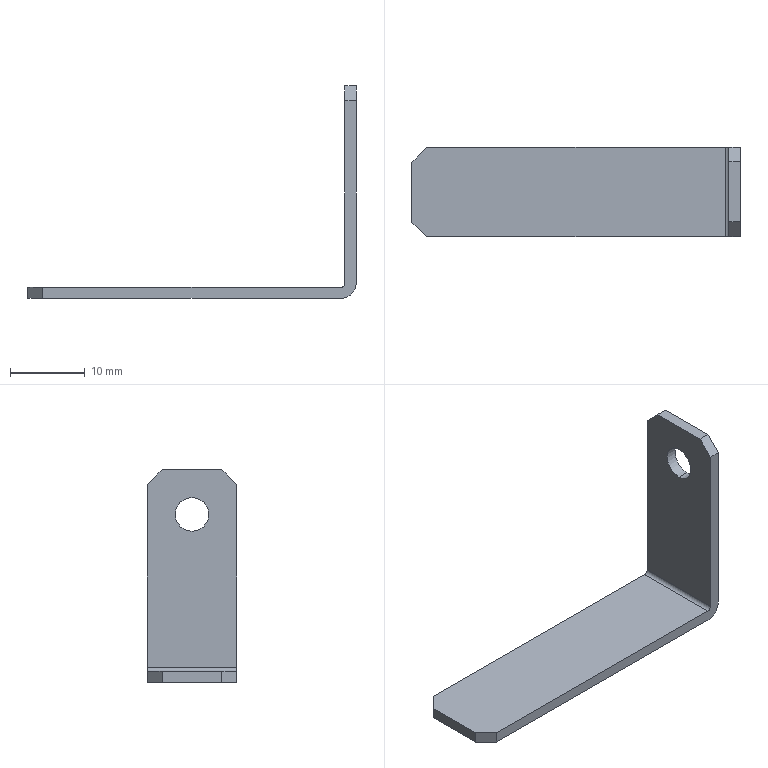Part | SolidWorks | features Fillet 2, Chamfer 1, Extrusion 1, ICE 1 | 1 solid | 16 faces | box 44 x 12 x 28.5 mm | volume 1232 mm3 | plane 12 | cylinder 4 | commonest cylinder face diameters 4.5 x2 1 x1 4 x1
STEP:
#1=CARTESIAN_POINT('',(-1.5,6.,-3.75));
#2=VERTEX_POINT('',#1);
#3=CARTESIAN_POINT('',(-1.5,6.,-8.25));
#4=VERTEX_POINT('',#3);
#5=CARTESIAN_POINT('',(-1.5,6.,-6.));
#6=DIRECTION('',(1.,0.,0.));
#7=DIRECTION('',(0.,0.,-1.));
#8=AXIS2_PLACEMENT_3D('',#5,#6,#7);
#9=CIRCLE('',#8,2.25);
#10=EDGE_CURVE('',#2,#4,#9,.T.);
#11=ORIENTED_EDGE('',*,*,#10,.F.);
#12=CARTESIAN_POINT('',(0.,6.,-3.75));
#13=VERTEX_POINT('',#12);
#14=CARTESIAN_POINT('',(-44.,6.,-3.75));
#15=DIRECTION('',(1.,0.,0.));
#16=VECTOR('',#15,1000.);
#17=LINE('',#14,#16);
#18=EDGE_CURVE('',#2,#13,#17,.T.);
#19=ORIENTED_EDGE('',*,*,#18,.T.);
#20=CARTESIAN_POINT('',(0.,6.,-8.25));
#21=VERTEX_POINT('',#20);
#22=CARTESIAN_POINT('',(0.,6.,-6.));
#23=DIRECTION('',(1.,0.,0.));
#24=DIRECTION('',(0.,0.,-1.));
#25=AXIS2_PLACEMENT_3D('',#22,#23,#24);
#26=CIRCLE('',#25,2.25);
#27=EDGE_CURVE('',#13,#21,#26,.T.);
#28=ORIENTED_EDGE('',*,*,#27,.T.);
#29=CARTESIAN_POINT('',(-44.,6.,-8.25));
#30=DIRECTION('',(1.,0.,0.));
#31=VECTOR('',#30,1000.);
#32=LINE('',#29,#31);
#33=EDGE_CURVE('',#4,#21,#32,.T.);
#34=ORIENTED_EDGE('',*,*,#33,.F.);
#35=EDGE_LOOP('',(#11,#19,#28,#34));
#36=FACE_OUTER_BOUND('',#35,.T.);
#37=CARTESIAN_POINT('',(-44.,6.,-6.));
#38=DIRECTION('',(1.,0.,0.));
#39=DIRECTION('',(0.,0.,-1.));
#40=AXIS2_PLACEMENT_3D('',#37,#38,#39);
#41=CYLINDRICAL_SURFACE('',#40,2.25);
#42=ADVANCED_FACE('',(#36),#41,.F.);
#43=CARTESIAN_POINT('',(0.,6.,-6.));
#44=DIRECTION('',(1.,0.,0.));
#45=DIRECTION('',(0.,0.,-1.));
#46=AXIS2_PLACEMENT_3D('',#43,#44,#45);
#47=CIRCLE('',#46,2.25);
#48=EDGE_CURVE('',#21,#13,#47,.T.);
#49=ORIENTED_EDGE('',*,*,#48,.F.);
#50=ORIENTED_EDGE('',*,*,#27,.F.);
#51=EDGE_LOOP('',(#49,#50));
#52=FACE_BOUND('',#51,.T.);
#53=CARTESIAN_POINT('',(0.,0.,-2.));
#54=VERTEX_POINT('',#53);
#55=CARTESIAN_POINT('',(0.,0.,-26.5));
#56=VERTEX_POINT('',#55);
#57=CARTESIAN_POINT('',(0.,0.,0.));
#58=DIRECTION('',(0.,0.,-1.));
#59=VECTOR('',#58,1000.);
#60=LINE('',#57,#59);
#61=EDGE_CURVE('',#54,#56,#60,.T.);
#62=ORIENTED_EDGE('',*,*,#61,.T.);
#63=CARTESIAN_POINT('',(0.,12.,-26.5));
#64=VERTEX_POINT('',#63);
#65=CARTESIAN_POINT('',(0.,12.,-26.5));
#66=DIRECTION('',(0.,1.,0.));
#67=VECTOR('',#66,1000.);
#68=LINE('',#65,#67);
#69=EDGE_CURVE('',#56,#64,#68,.T.);
#70=ORIENTED_EDGE('',*,*,#69,.T.);
#71=CARTESIAN_POINT('',(0.,12.,-2.));
#72=VERTEX_POINT('',#71);
#73=CARTESIAN_POINT('',(0.,12.,0.));
#74=DIRECTION('',(0.,0.,-1.));
#75=VECTOR('',#74,1000.);
#76=LINE('',#73,#75);
#77=EDGE_CURVE('',#72,#64,#76,.T.);
#78=ORIENTED_EDGE('',*,*,#77,.F.);
#79=CARTESIAN_POINT('',(0.,10.,0.));
#80=VERTEX_POINT('',#79);
#81=CARTESIAN_POINT('',(0.,12.,-2.));
#82=DIRECTION('',(0.,-0.7071,0.7071));
#83=VECTOR('',#82,1000.);
#84=LINE('',#81,#83);
#85=EDGE_CURVE('',#72,#80,#84,.T.);
#86=ORIENTED_EDGE('',*,*,#85,.T.);
#87=CARTESIAN_POINT('',(0.,2.,0.));
#88=VERTEX_POINT('',#87);
#89=CARTESIAN_POINT('',(0.,12.,0.));
#90=DIRECTION('',(0.,-1.,0.));
#91=VECTOR('',#90,1000.);
#92=LINE('',#89,#91);
#93=EDGE_CURVE('',#80,#88,#92,.T.);
#94=ORIENTED_EDGE('',*,*,#93,.T.);
#95=CARTESIAN_POINT('',(0.,2.,0.));
#96=DIRECTION('',(0.,-0.7071,-0.7071));
#97=VECTOR('',#96,1000.);
#98=LINE('',#95,#97);
#99=EDGE_CURVE('',#88,#54,#98,.T.);
#100=ORIENTED_EDGE('',*,*,#99,.T.);
#101=EDGE_LOOP('',(#62,#70,#78,#86,#94,#100));
#102=FACE_OUTER_BOUND('',#101,.T.);
#103=CARTESIAN_POINT('',(0.,12.,0.));
#104=DIRECTION('',(-1.,0.,0.));
#105=DIRECTION('',(0.,0.,1.));
#106=AXIS2_PLACEMENT_3D('',#103,#104,#105);
#107=PLANE('',#106);
#108=ADVANCED_FACE('',(#52,#102),#107,.F.);
#109=CARTESIAN_POINT('',(-2.,12.,-28.5));
#110=VERTEX_POINT('',#109);
#111=CARTESIAN_POINT('',(-42.,12.,-28.5));
#112=VERTEX_POINT('',#111);
#113=CARTESIAN_POINT('',(0.,12.,-28.5));
#114=DIRECTION('',(-1.,0.,0.));
#115=VECTOR('',#114,1000.);
#116=LINE('',#113,#115);
#117=EDGE_CURVE('',#110,#112,#116,.T.);
#118=ORIENTED_EDGE('',*,*,#117,.F.);
#119=CARTESIAN_POINT('',(-2.,0.,-28.5));
#120=VERTEX_POINT('',#119);
#121=CARTESIAN_POINT('',(-2.,12.,-28.5));
#122=DIRECTION('',(0.,-1.,0.));
#123=VECTOR('',#122,1000.);
#124=LINE('',#121,#123);
#125=EDGE_CURVE('',#110,#120,#124,.T.);
#126=ORIENTED_EDGE('',*,*,#125,.T.);
#127=CARTESIAN_POINT('',(-42.,0.,-28.5));
#128=VERTEX_POINT('',#127);
#129=CARTESIAN_POINT('',(0.,0.,-28.5));
#130=DIRECTION('',(-1.,0.,0.));
#131=VECTOR('',#130,1000.);
#132=LINE('',#129,#131);
#133=EDGE_CURVE('',#120,#128,#132,.T.);
#134=ORIENTED_EDGE('',*,*,#133,.T.);
#135=CARTESIAN_POINT('',(-44.,2.,-28.5));
#136=VERTEX_POINT('',#135);
#137=CARTESIAN_POINT('',(-44.,2.,-28.5));
#138=DIRECTION('',(-0.7071,0.7071,0.));
#139=VECTOR('',#138,1000.);
#140=LINE('',#137,#139);
#141=EDGE_CURVE('',#128,#136,#140,.T.);
#142=ORIENTED_EDGE('',*,*,#141,.T.);
#143=CARTESIAN_POINT('',(-44.,10.,-28.5));
#144=VERTEX_POINT('',#143);
#145=CARTESIAN_POINT('',(-44.,12.,-28.5));
#146=DIRECTION('',(0.,-1.,0.));
#147=VECTOR('',#146,1000.);
#148=LINE('',#145,#147);
#149=EDGE_CURVE('',#144,#136,#148,.T.);
#150=ORIENTED_EDGE('',*,*,#149,.F.);
#151=CARTESIAN_POINT('',(-42.,12.,-28.5));
#152=DIRECTION('',(0.7071,0.7071,0.));
#153=VECTOR('',#152,1000.);
#154=LINE('',#151,#153);
#155=EDGE_CURVE('',#144,#112,#154,.T.);
#156=ORIENTED_EDGE('',*,*,#155,.T.);
#157=EDGE_LOOP('',(#118,#126,#134,#142,#150,#156));
#158=FACE_OUTER_BOUND('',#157,.T.);
#159=CARTESIAN_POINT('',(0.,12.,-28.5));
#160=DIRECTION('',(0.,0.,1.));
#161=DIRECTION('',(1.,0.,0.));
#162=AXIS2_PLACEMENT_3D('',#159,#160,#161);
#163=PLANE('',#162);
#164=ADVANCED_FACE('',(#158),#163,.F.);
#165=ORIENTED_EDGE('',*,*,#149,.T.);
#166=CARTESIAN_POINT('',(-44.,2.,-27.));
#167=VERTEX_POINT('',#166);
#168=CARTESIAN_POINT('',(-44.,2.,-27.));
#169=DIRECTION('',(0.,0.,1.));
#170=VECTOR('',#169,1000.);
#171=LINE('',#168,#170);
#172=EDGE_CURVE('',#136,#167,#171,.T.);
#173=ORIENTED_EDGE('',*,*,#172,.T.);
#174=CARTESIAN_POINT('',(-44.,10.,-27.));
#175=VERTEX_POINT('',#174);
#176=CARTESIAN_POINT('',(-44.,12.,-27.));
#177=DIRECTION('',(0.,-1.,0.));
#178=VECTOR('',#177,1000.);
#179=LINE('',#176,#178);
#180=EDGE_CURVE('',#175,#167,#179,.T.);
#181=ORIENTED_EDGE('',*,*,#180,.F.);
#182=CARTESIAN_POINT('',(-44.,10.,-28.5));
#183=DIRECTION('',(0.,0.,-1.));
#184=VECTOR('',#183,1000.);
#185=LINE('',#182,#184);
#186=EDGE_CURVE('',#175,#144,#185,.T.);
#187=ORIENTED_EDGE('',*,*,#186,.T.);
#188=EDGE_LOOP('',(#165,#173,#181,#187));
#189=FACE_OUTER_BOUND('',#188,.T.);
#190=CARTESIAN_POINT('',(-44.,12.,-27.));
#191=DIRECTION('',(1.,0.,0.));
#192=DIRECTION('',(0.,0.,-1.));
#193=AXIS2_PLACEMENT_3D('',#190,#191,#192);
#194=PLANE('',#193);
#195=ADVANCED_FACE('',(#189),#194,.F.);
#196=CARTESIAN_POINT('',(-42.,0.,-27.));
#197=VERTEX_POINT('',#196);
#198=CARTESIAN_POINT('',(-2.,0.,-27.));
#199=VERTEX_POINT('',#198);
#200=CARTESIAN_POINT('',(-44.,0.,-27.));
#201=DIRECTION('',(1.,0.,0.));
#202=VECTOR('',#201,1000.);
#203=LINE('',#200,#202);
#204=EDGE_CURVE('',#197,#199,#203,.T.);
#205=ORIENTED_EDGE('',*,*,#204,.T.);
#206=CARTESIAN_POINT('',(-2.,12.,-27.));
#207=VERTEX_POINT('',#206);
#208=CARTESIAN_POINT('',(-2.,12.,-27.));
#209=DIRECTION('',(0.,1.,0.));
#210=VECTOR('',#209,1000.);
#211=LINE('',#208,#210);
#212=EDGE_CURVE('',#199,#207,#211,.T.);
#213=ORIENTED_EDGE('',*,*,#212,.T.);
#214=CARTESIAN_POINT('',(-42.,12.,-27.));
#215=VERTEX_POINT('',#214);
#216=CARTESIAN_POINT('',(-44.,12.,-27.));
#217=DIRECTION('',(1.,0.,0.));
#218=VECTOR('',#217,1000.);
#219=LINE('',#216,#218);
#220=EDGE_CURVE('',#215,#207,#219,.T.);
#221=ORIENTED_EDGE('',*,*,#220,.F.);
#222=CARTESIAN_POINT('',(-42.,12.,-27.));
#223=DIRECTION('',(-0.7071,-0.7071,0.));
#224=VECTOR('',#223,1000.);
#225=LINE('',#222,#224);
#226=EDGE_CURVE('',#215,#175,#225,.T.);
#227=ORIENTED_EDGE('',*,*,#226,.T.);
#228=ORIENTED_EDGE('',*,*,#180,.T.);
#229=CARTESIAN_POINT('',(-44.,2.,-27.));
#230=DIRECTION('',(0.7071,-0.7071,0.));
#231=VECTOR('',#230,1000.);
#232=LINE('',#229,#231);
#233=EDGE_CURVE('',#167,#197,#232,.T.);
#234=ORIENTED_EDGE('',*,*,#233,.T.);
#235=EDGE_LOOP('',(#205,#213,#221,#227,#228,#234));
#236=FACE_OUTER_BOUND('',#235,.T.);
#237=CARTESIAN_POINT('',(-44.,12.,-27.));
#238=DIRECTION('',(0.,0.,-1.));
#239=DIRECTION('',(-1.,0.,0.));
#240=AXIS2_PLACEMENT_3D('',#237,#238,#239);
#241=PLANE('',#240);
#242=ADVANCED_FACE('',(#236),#241,.F.);
#243=CARTESIAN_POINT('',(-1.5,6.,-6.));
#244=DIRECTION('',(1.,0.,0.));
#245=DIRECTION('',(0.,0.,-1.));
#246=AXIS2_PLACEMENT_3D('',#243,#244,#245);
#247=CIRCLE('',#246,2.25);
#248=EDGE_CURVE('',#4,#2,#247,.T.);
#249=ORIENTED_EDGE('',*,*,#248,.T.);
#250=ORIENTED_EDGE('',*,*,#10,.T.);
#251=EDGE_LOOP('',(#249,#250));
#252=FACE_BOUND('',#251,.T.);
#253=CARTESIAN_POINT('',(-1.5,12.,-26.5));
#254=VERTEX_POINT('',#253);
#255=CARTESIAN_POINT('',(-1.5,12.,-2.));
#256=VERTEX_POINT('',#255);
#257=CARTESIAN_POINT('',(-1.5,12.,0.));
#258=DIRECTION('',(0.,0.,1.));
#259=VECTOR('',#258,1000.);
#260=LINE('',#257,#259);
#261=EDGE_CURVE('',#254,#256,#260,.T.);
#262=ORIENTED_EDGE('',*,*,#261,.F.);
#263=CARTESIAN_POINT('',(-1.5,0.,-26.5));
#264=VERTEX_POINT('',#263);
#265=CARTESIAN_POINT('',(-1.5,0.,-26.5));
#266=DIRECTION('',(0.,-1.,0.));
#267=VECTOR('',#266,1000.);
#268=LINE('',#265,#267);
#269=EDGE_CURVE('',#254,#264,#268,.T.);
#270=ORIENTED_EDGE('',*,*,#269,.T.);
#271=CARTESIAN_POINT('',(-1.5,0.,-2.));
#272=VERTEX_POINT('',#271);
#273=CARTESIAN_POINT('',(-1.5,0.,0.));
#274=DIRECTION('',(0.,0.,1.));
#275=VECTOR('',#274,1000.);
#276=LINE('',#273,#275);
#277=EDGE_CURVE('',#264,#272,#276,.T.);
#278=ORIENTED_EDGE('',*,*,#277,.T.);
#279=CARTESIAN_POINT('',(-1.5,2.,0.));
#280=VERTEX_POINT('',#279);
#281=CARTESIAN_POINT('',(-1.5,2.,0.));
#282=DIRECTION('',(0.,0.7071,0.7071));
#283=VECTOR('',#282,1000.);
#284=LINE('',#281,#283);
#285=EDGE_CURVE('',#272,#280,#284,.T.);
#286=ORIENTED_EDGE('',*,*,#285,.T.);
#287=CARTESIAN_POINT('',(-1.5,10.,0.));
#288=VERTEX_POINT('',#287);
#289=CARTESIAN_POINT('',(-1.5,12.,0.));
#290=DIRECTION('',(0.,-1.,0.));
#291=VECTOR('',#290,1000.);
#292=LINE('',#289,#291);
#293=EDGE_CURVE('',#288,#280,#292,.T.);
#294=ORIENTED_EDGE('',*,*,#293,.F.);
#295=CARTESIAN_POINT('',(-1.5,12.,-2.));
#296=DIRECTION('',(0.,0.7071,-0.7071));
#297=VECTOR('',#296,1000.);
#298=LINE('',#295,#297);
#299=EDGE_CURVE('',#288,#256,#298,.T.);
#300=ORIENTED_EDGE('',*,*,#299,.T.);
#301=EDGE_LOOP('',(#262,#270,#278,#286,#294,#300));
#302=FACE_OUTER_BOUND('',#301,.T.);
#303=CARTESIAN_POINT('',(-1.5,12.,0.));
#304=DIRECTION('',(1.,0.,0.));
#305=DIRECTION('',(0.,0.,-1.));
#306=AXIS2_PLACEMENT_3D('',#303,#304,#305);
#307=PLANE('',#306);
#308=ADVANCED_FACE('',(#252,#302),#307,.F.);
#309=ORIENTED_EDGE('',*,*,#293,.T.);
#310=CARTESIAN_POINT('',(0.,2.,0.));
#311=DIRECTION('',(1.,0.,0.));
#312=VECTOR('',#311,1000.);
#313=LINE('',#310,#312);
#314=EDGE_CURVE('',#280,#88,#313,.T.);
#315=ORIENTED_EDGE('',*,*,#314,.T.);
#316=ORIENTED_EDGE('',*,*,#93,.F.);
#317=CARTESIAN_POINT('',(-1.5,10.,0.));
#318=DIRECTION('',(-1.,0.,0.));
#319=VECTOR('',#318,1000.);
#320=LINE('',#317,#319);
#321=EDGE_CURVE('',#80,#288,#320,.T.);
#322=ORIENTED_EDGE('',*,*,#321,.T.);
#323=EDGE_LOOP('',(#309,#315,#316,#322));
#324=FACE_OUTER_BOUND('',#323,.T.);
#325=CARTESIAN_POINT('',(0.,12.,0.));
#326=DIRECTION('',(0.,0.,-1.));
#327=DIRECTION('',(-1.,0.,0.));
#328=AXIS2_PLACEMENT_3D('',#325,#326,#327);
#329=PLANE('',#328);
#330=ADVANCED_FACE('',(#324),#329,.F.);
#331=ORIENTED_EDGE('',*,*,#77,.T.);
#332=CARTESIAN_POINT('',(-2.,12.,-26.5));
#333=DIRECTION('',(0.,1.,0.));
#334=DIRECTION('',(0.,0.,1.));
#335=AXIS2_PLACEMENT_3D('',#332,#333,#334);
#336=CIRCLE('',#335,2.);
#337=EDGE_CURVE('',#64,#110,#336,.T.);
#338=ORIENTED_EDGE('',*,*,#337,.T.);
#339=ORIENTED_EDGE('',*,*,#117,.T.);
#340=CARTESIAN_POINT('',(-42.,12.,-27.));
#341=DIRECTION('',(0.,0.,1.));
#342=VECTOR('',#341,1000.);
#343=LINE('',#340,#342);
#344=EDGE_CURVE('',#112,#215,#343,.T.);
#345=ORIENTED_EDGE('',*,*,#344,.T.);
#346=ORIENTED_EDGE('',*,*,#220,.T.);
#347=CARTESIAN_POINT('',(-2.,12.,-26.5));
#348=DIRECTION('',(0.,-1.,0.));
#349=DIRECTION('',(0.,0.,1.));
#350=AXIS2_PLACEMENT_3D('',#347,#348,#349);
#351=CIRCLE('',#350,0.5);
#352=EDGE_CURVE('',#207,#254,#351,.T.);
#353=ORIENTED_EDGE('',*,*,#352,.T.);
#354=ORIENTED_EDGE('',*,*,#261,.T.);
#355=CARTESIAN_POINT('',(0.,12.,-2.));
#356=DIRECTION('',(1.,0.,0.));
#357=VECTOR('',#356,1000.);
#358=LINE('',#355,#357);
#359=EDGE_CURVE('',#256,#72,#358,.T.);
#360=ORIENTED_EDGE('',*,*,#359,.T.);
#361=EDGE_LOOP('',(#331,#338,#339,#345,#346,#353,#354,#360));
#362=FACE_OUTER_BOUND('',#361,.T.);
#363=CARTESIAN_POINT('',(0.,12.,0.));
#364=DIRECTION('',(0.,1.,0.));
#365=DIRECTION('',(0.,0.,1.));
#366=AXIS2_PLACEMENT_3D('',#363,#364,#365);
#367=PLANE('',#366);
#368=ADVANCED_FACE('',(#362),#367,.T.);
#369=ORIENTED_EDGE('',*,*,#133,.F.);
#370=CARTESIAN_POINT('',(-2.,0.,-26.5));
#371=DIRECTION('',(0.,-1.,0.));
#372=DIRECTION('',(0.,0.,1.));
#373=AXIS2_PLACEMENT_3D('',#370,#371,#372);
#374=CIRCLE('',#373,2.);
#375=EDGE_CURVE('',#120,#56,#374,.T.);
#376=ORIENTED_EDGE('',*,*,#375,.T.);
#377=ORIENTED_EDGE('',*,*,#61,.F.);
#378=CARTESIAN_POINT('',(0.,0.,-2.));
#379=DIRECTION('',(-1.,0.,0.));
#380=VECTOR('',#379,1000.);
#381=LINE('',#378,#380);
#382=EDGE_CURVE('',#54,#272,#381,.T.);
#383=ORIENTED_EDGE('',*,*,#382,.T.);
#384=ORIENTED_EDGE('',*,*,#277,.F.);
#385=CARTESIAN_POINT('',(-2.,0.,-26.5));
#386=DIRECTION('',(0.,1.,0.));
#387=DIRECTION('',(0.,0.,1.));
#388=AXIS2_PLACEMENT_3D('',#385,#386,#387);
#389=CIRCLE('',#388,0.5);
#390=EDGE_CURVE('',#264,#199,#389,.T.);
#391=ORIENTED_EDGE('',*,*,#390,.T.);
#392=ORIENTED_EDGE('',*,*,#204,.F.);
#393=CARTESIAN_POINT('',(-42.,0.,0.));
#394=DIRECTION('',(0.,0.,-1.));
#395=VECTOR('',#394,1000.);
#396=LINE('',#393,#395);
#397=EDGE_CURVE('',#197,#128,#396,.T.);
#398=ORIENTED_EDGE('',*,*,#397,.T.);
#399=EDGE_LOOP('',(#369,#376,#377,#383,#384,#391,#392,#398));
#400=FACE_OUTER_BOUND('',#399,.T.);
#401=CARTESIAN_POINT('',(0.,0.,0.));
#402=DIRECTION('',(0.,1.,0.));
#403=DIRECTION('',(0.,0.,1.));
#404=AXIS2_PLACEMENT_3D('',#401,#402,#403);
#405=PLANE('',#404);
#406=ADVANCED_FACE('',(#400),#405,.F.);
#407=ORIENTED_EDGE('',*,*,#18,.F.);
#408=ORIENTED_EDGE('',*,*,#248,.F.);
#409=ORIENTED_EDGE('',*,*,#33,.T.);
#410=ORIENTED_EDGE('',*,*,#48,.T.);
#411=EDGE_LOOP('',(#407,#408,#409,#410));
#412=FACE_OUTER_BOUND('',#411,.T.);
#413=CARTESIAN_POINT('',(-44.,6.,-6.));
#414=DIRECTION('',(1.,0.,0.));
#415=DIRECTION('',(0.,0.,-1.));
#416=AXIS2_PLACEMENT_3D('',#413,#414,#415);
#417=CYLINDRICAL_SURFACE('',#416,2.25);
#418=ADVANCED_FACE('',(#412),#417,.F.);
#419=ORIENTED_EDGE('',*,*,#141,.F.);
#420=ORIENTED_EDGE('',*,*,#397,.F.);
#421=ORIENTED_EDGE('',*,*,#233,.F.);
#422=ORIENTED_EDGE('',*,*,#172,.F.);
#423=EDGE_LOOP('',(#419,#420,#421,#422));
#424=FACE_OUTER_BOUND('',#423,.T.);
#425=CARTESIAN_POINT('',(-44.,2.,-27.));
#426=DIRECTION('',(0.7071,0.7071,0.));
#427=DIRECTION('',(0.,0.,1.));
#428=AXIS2_PLACEMENT_3D('',#425,#426,#427);
#429=PLANE('',#428);
#430=ADVANCED_FACE('',(#424),#429,.F.);
#431=ORIENTED_EDGE('',*,*,#155,.F.);
#432=ORIENTED_EDGE('',*,*,#186,.F.);
#433=ORIENTED_EDGE('',*,*,#226,.F.);
#434=ORIENTED_EDGE('',*,*,#344,.F.);
#435=EDGE_LOOP('',(#431,#432,#433,#434));
#436=FACE_OUTER_BOUND('',#435,.T.);
#437=CARTESIAN_POINT('',(-42.,12.,0.));
#438=DIRECTION('',(-0.7071,0.7071,0.));
#439=DIRECTION('',(0.,0.,-1.));
#440=AXIS2_PLACEMENT_3D('',#437,#438,#439);
#441=PLANE('',#440);
#442=ADVANCED_FACE('',(#436),#441,.T.);
#443=ORIENTED_EDGE('',*,*,#285,.F.);
#444=ORIENTED_EDGE('',*,*,#382,.F.);
#445=ORIENTED_EDGE('',*,*,#99,.F.);
#446=ORIENTED_EDGE('',*,*,#314,.F.);
#447=EDGE_LOOP('',(#443,#444,#445,#446));
#448=FACE_OUTER_BOUND('',#447,.T.);
#449=CARTESIAN_POINT('',(0.,2.,0.));
#450=DIRECTION('',(0.,0.7071,-0.7071));
#451=DIRECTION('',(1.,0.,0.));
#452=AXIS2_PLACEMENT_3D('',#449,#450,#451);
#453=PLANE('',#452);
#454=ADVANCED_FACE('',(#448),#453,.F.);
#455=ORIENTED_EDGE('',*,*,#299,.F.);
#456=ORIENTED_EDGE('',*,*,#321,.F.);
#457=ORIENTED_EDGE('',*,*,#85,.F.);
#458=ORIENTED_EDGE('',*,*,#359,.F.);
#459=EDGE_LOOP('',(#455,#456,#457,#458));
#460=FACE_OUTER_BOUND('',#459,.T.);
#461=CARTESIAN_POINT('',(0.,12.,-2.));
#462=DIRECTION('',(0.,0.7071,0.7071));
#463=DIRECTION('',(-1.,0.,0.));
#464=AXIS2_PLACEMENT_3D('',#461,#462,#463);
#465=PLANE('',#464);
#466=ADVANCED_FACE('',(#460),#465,.T.);
#467=ORIENTED_EDGE('',*,*,#337,.F.);
#468=ORIENTED_EDGE('',*,*,#69,.F.);
#469=ORIENTED_EDGE('',*,*,#375,.F.);
#470=ORIENTED_EDGE('',*,*,#125,.F.);
#471=EDGE_LOOP('',(#467,#468,#469,#470));
#472=FACE_OUTER_BOUND('',#471,.T.);
#473=CARTESIAN_POINT('',(-2.,12.,-26.5));
#474=DIRECTION('',(0.,-1.,0.));
#475=DIRECTION('',(0.,0.,-1.));
#476=AXIS2_PLACEMENT_3D('',#473,#474,#475);
#477=CYLINDRICAL_SURFACE('',#476,2.);
#478=ADVANCED_FACE('',(#472),#477,.T.);
#479=ORIENTED_EDGE('',*,*,#352,.F.);
#480=ORIENTED_EDGE('',*,*,#212,.F.);
#481=ORIENTED_EDGE('',*,*,#390,.F.);
#482=ORIENTED_EDGE('',*,*,#269,.F.);
#483=EDGE_LOOP('',(#479,#480,#481,#482));
#484=FACE_OUTER_BOUND('',#483,.T.);
#485=CARTESIAN_POINT('',(-2.,12.,-26.5));
#486=DIRECTION('',(0.,1.,0.));
#487=DIRECTION('',(0.,0.,1.));
#488=AXIS2_PLACEMENT_3D('',#485,#486,#487);
#489=CYLINDRICAL_SURFACE('',#488,0.5);
#490=ADVANCED_FACE('',(#484),#489,.F.);
#491=CLOSED_SHELL('',(#42,#108,#164,#195,#242,#308,#330,#368,#406,#418,#430,#442,#454,#466,#478,#490));
#492=MANIFOLD_SOLID_BREP('',#491);
#493=CARTESIAN_POINT('',(0.,0.,0.));
#494=DIRECTION('',(0.,0.,1.));
#495=DIRECTION('',(1.,0.,0.));
#496=AXIS2_PLACEMENT_3D('',#493,#494,#495);
#497=(LENGTH_UNIT()NAMED_UNIT(*)SI_UNIT(.MILLI.,.METRE.));
#498=UNCERTAINTY_MEASURE_WITH_UNIT(LENGTH_MEASURE(0.00001),#497,'','');
#499=(NAMED_UNIT(*)PLANE_ANGLE_UNIT()SI_UNIT($,.RADIAN.));
#500=(NAMED_UNIT(*)SI_UNIT($,.STERADIAN.)SOLID_ANGLE_UNIT());
#501=(GEOMETRIC_REPRESENTATION_CONTEXT(3)GLOBAL_UNCERTAINTY_ASSIGNED_CONTEXT((#498))GLOBAL_UNIT_ASSIGNED_CONTEXT((#497,#499,#500))REPRESENTATION_CONTEXT('',''));
#502=ADVANCED_BREP_SHAPE_REPRESENTATION('',(#492,#496),#501);